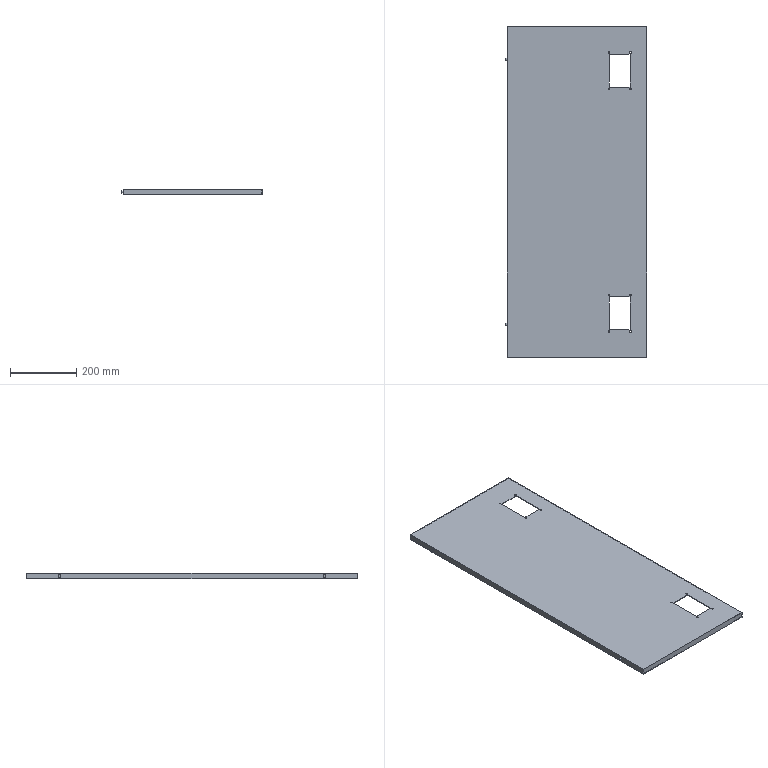Part | SolidWorks | features BaseBody 1 | 1 solid | 54 faces | box 426 x 996 x 18 mm | volume 976577 mm3 | cylinder 28 | plane 26 | commonest cylinder face diameters 5 x16 2.5 x8 8 x4